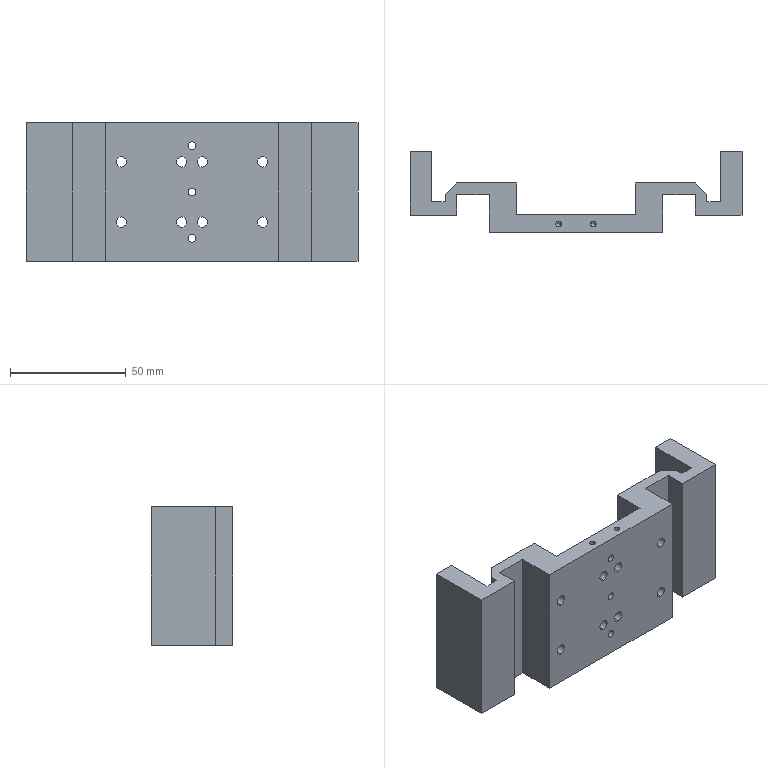Part | SolidWorks | features HoleWzd 8, MirrorPattern 5, ICE 3, Chamfer 1, Extrusion 1, LPattern 1 | 1 solid | 122 faces | box 143.4 x 35.1 x 60 mm | volume 99066 mm3 | cylinder 62 | plane 36 | cone 24 | commonest cylinder face diameters 4.5 x16 8 x16 3.3 x14 2.5 x12 6 x4